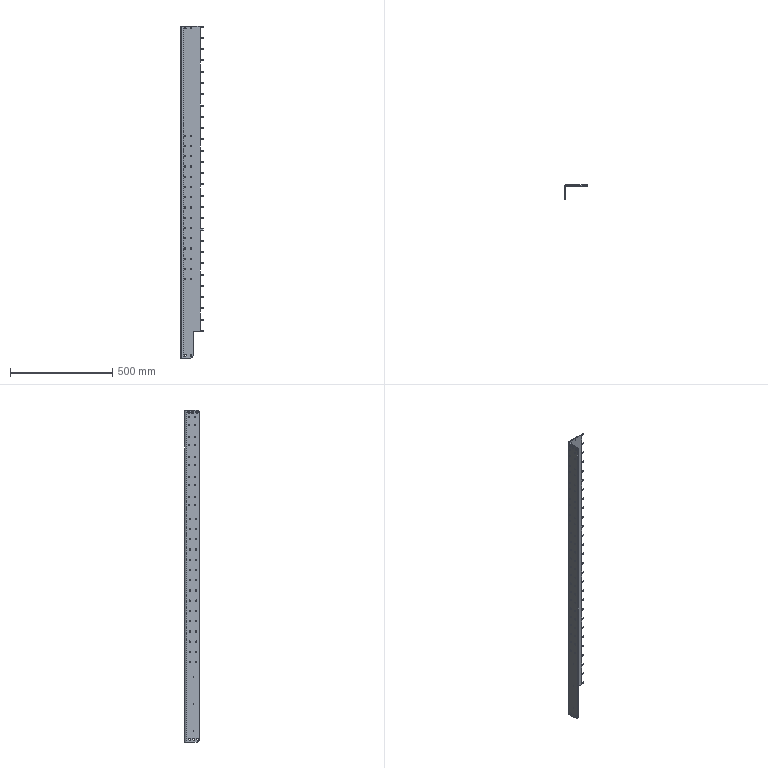Part | SolidWorks | features HoleWzd 8, MoveFace 3, Fillet 2, LPattern 2, Cut 1, Extrusion 1, ICE 1 | 1 solid | 335 faces | box 110 x 70 x 1620 mm | volume 1267846 mm3 | cylinder 197 | plane 128 | cone 10 | commonest cylinder face diameters 6.8 x120 5.5 x40 5.8 x25 4.2 x6 20 x4 16 x2